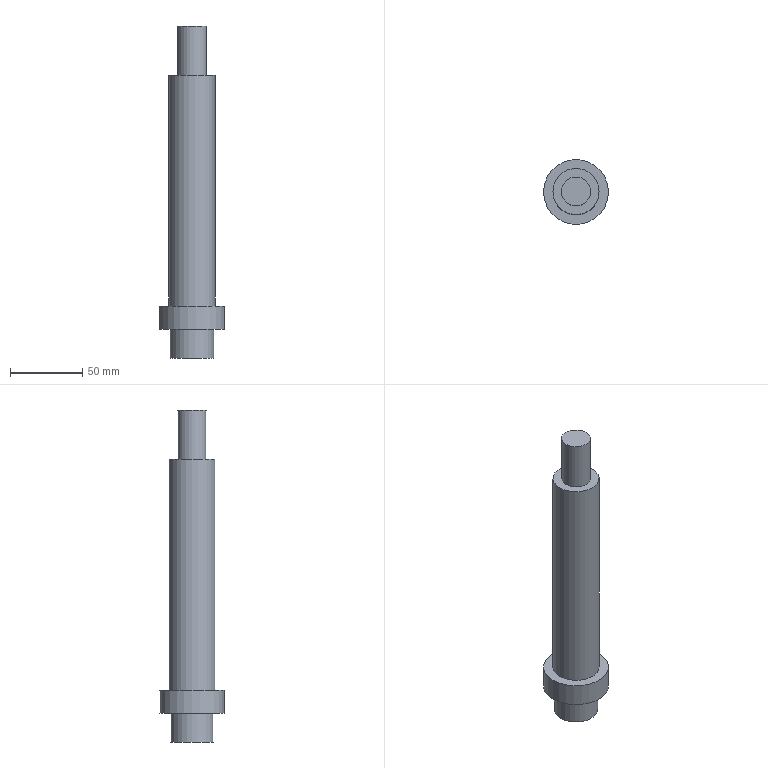Part | NX | features solid 2 | 1 solid | 9 faces | box 45 x 45 x 230 mm | volume 178945 mm3 | plane 5 | cylinder 4 | commonest cylinder face diameters 20 x1 30 x1 32 x1 45 x1
STEP:
#1=CARTESIAN_POINT('',(-305.,-95.,350.));
#2=VERTEX_POINT('',#1);
#3=CARTESIAN_POINT('',(-315.,-95.,350.));
#4=DIRECTION('',(0.,0.,1.));
#5=DIRECTION('',(1.,0.,0.));
#6=AXIS2_PLACEMENT_3D('',#3,#4,#5);
#7=CIRCLE('',#6,10.);
#8=EDGE_CURVE('',#2,#2,#7,.F.);
#9=ORIENTED_EDGE('',*,*,#8,.T.);
#10=EDGE_LOOP('',(#9));
#11=FACE_BOUND('',#10,.T.);
#12=CARTESIAN_POINT('',(-299.,-95.,350.));
#13=VERTEX_POINT('',#12);
#14=CARTESIAN_POINT('',(-315.,-95.,350.));
#15=DIRECTION('',(0.,0.,1.));
#16=DIRECTION('',(1.,0.,0.));
#17=AXIS2_PLACEMENT_3D('',#14,#15,#16);
#18=CIRCLE('',#17,16.);
#19=EDGE_CURVE('',#13,#13,#18,.T.);
#20=ORIENTED_EDGE('',*,*,#19,.T.);
#21=EDGE_LOOP('',(#20));
#22=FACE_BOUND('',#21,.T.);
#23=CARTESIAN_POINT('',(-315.,-95.,350.));
#24=DIRECTION('',(0.,0.,1.));
#25=DIRECTION('',(-1.,0.,0.));
#26=AXIS2_PLACEMENT_3D('',#23,#24,#25);
#27=PLANE('',#26);
#28=ADVANCED_FACE('',(#11,#22),#27,.T.);
#29=CARTESIAN_POINT('',(-331.,-95.,190.));
#30=VERTEX_POINT('',#29);
#31=CARTESIAN_POINT('',(-315.,-95.,190.));
#32=DIRECTION('',(0.,0.,-1.));
#33=DIRECTION('',(-1.,0.,0.));
#34=AXIS2_PLACEMENT_3D('',#31,#32,#33);
#35=CIRCLE('',#34,16.);
#36=EDGE_CURVE('',#30,#30,#35,.F.);
#37=ORIENTED_EDGE('',*,*,#36,.T.);
#38=EDGE_LOOP('',(#37));
#39=FACE_BOUND('',#38,.T.);
#40=ORIENTED_EDGE('',*,*,#19,.F.);
#41=EDGE_LOOP('',(#40));
#42=FACE_BOUND('',#41,.T.);
#43=CARTESIAN_POINT('',(-315.,-95.,430.));
#44=DIRECTION('',(0.,0.,-1.));
#45=DIRECTION('',(1.,0.,0.));
#46=AXIS2_PLACEMENT_3D('',#43,#44,#45);
#47=CYLINDRICAL_SURFACE('',#46,16.);
#48=ADVANCED_FACE('',(#39,#42),#47,.T.);
#49=CARTESIAN_POINT('',(-305.,-95.,384.));
#50=VERTEX_POINT('',#49);
#51=CARTESIAN_POINT('',(-315.,-95.,384.));
#52=DIRECTION('',(0.,0.,1.));
#53=DIRECTION('',(1.,0.,0.));
#54=AXIS2_PLACEMENT_3D('',#51,#52,#53);
#55=CIRCLE('',#54,10.);
#56=EDGE_CURVE('',#50,#50,#55,.T.);
#57=ORIENTED_EDGE('',*,*,#56,.T.);
#58=EDGE_LOOP('',(#57));
#59=FACE_BOUND('',#58,.T.);
#60=CARTESIAN_POINT('',(-315.,-95.,384.));
#61=DIRECTION('',(0.,0.,1.));
#62=DIRECTION('',(-1.,0.,0.));
#63=AXIS2_PLACEMENT_3D('',#60,#61,#62);
#64=PLANE('',#63);
#65=ADVANCED_FACE('',(#59),#64,.T.);
#66=ORIENTED_EDGE('',*,*,#56,.F.);
#67=EDGE_LOOP('',(#66));
#68=FACE_BOUND('',#67,.T.);
#69=ORIENTED_EDGE('',*,*,#8,.F.);
#70=EDGE_LOOP('',(#69));
#71=FACE_BOUND('',#70,.T.);
#72=CARTESIAN_POINT('',(-315.,-95.,430.));
#73=DIRECTION('',(0.,0.,1.));
#74=DIRECTION('',(-1.,0.,0.));
#75=AXIS2_PLACEMENT_3D('',#72,#73,#74);
#76=CYLINDRICAL_SURFACE('',#75,10.);
#77=ADVANCED_FACE('',(#68,#71),#76,.T.);
#78=CARTESIAN_POINT('',(-300.,-95.,174.));
#79=VERTEX_POINT('',#78);
#80=CARTESIAN_POINT('',(-315.,-95.,174.));
#81=DIRECTION('',(0.,0.,1.));
#82=DIRECTION('',(1.,0.,0.));
#83=AXIS2_PLACEMENT_3D('',#80,#81,#82);
#84=CIRCLE('',#83,15.);
#85=EDGE_CURVE('',#79,#79,#84,.T.);
#86=ORIENTED_EDGE('',*,*,#85,.T.);
#87=EDGE_LOOP('',(#86));
#88=FACE_BOUND('',#87,.T.);
#89=CARTESIAN_POINT('',(-337.5,-95.,174.));
#90=VERTEX_POINT('',#89);
#91=CARTESIAN_POINT('',(-315.,-95.,174.));
#92=DIRECTION('',(0.,0.,-1.));
#93=DIRECTION('',(-1.,0.,0.));
#94=AXIS2_PLACEMENT_3D('',#91,#92,#93);
#95=CIRCLE('',#94,22.5);
#96=EDGE_CURVE('',#90,#90,#95,.T.);
#97=ORIENTED_EDGE('',*,*,#96,.T.);
#98=EDGE_LOOP('',(#97));
#99=FACE_BOUND('',#98,.T.);
#100=CARTESIAN_POINT('',(-315.,-95.,174.));
#101=DIRECTION('',(0.,0.,-1.));
#102=DIRECTION('',(1.,0.,0.));
#103=AXIS2_PLACEMENT_3D('',#100,#101,#102);
#104=PLANE('',#103);
#105=ADVANCED_FACE('',(#88,#99),#104,.T.);
#106=ORIENTED_EDGE('',*,*,#36,.F.);
#107=EDGE_LOOP('',(#106));
#108=FACE_BOUND('',#107,.T.);
#109=CARTESIAN_POINT('',(-292.5,-95.,190.));
#110=VERTEX_POINT('',#109);
#111=CARTESIAN_POINT('',(-315.,-95.,190.));
#112=DIRECTION('',(0.,0.,1.));
#113=DIRECTION('',(1.,0.,0.));
#114=AXIS2_PLACEMENT_3D('',#111,#112,#113);
#115=CIRCLE('',#114,22.5);
#116=EDGE_CURVE('',#110,#110,#115,.T.);
#117=ORIENTED_EDGE('',*,*,#116,.T.);
#118=EDGE_LOOP('',(#117));
#119=FACE_BOUND('',#118,.T.);
#120=CARTESIAN_POINT('',(-315.,-95.,190.));
#121=DIRECTION('',(0.,0.,1.));
#122=DIRECTION('',(-1.,0.,0.));
#123=AXIS2_PLACEMENT_3D('',#120,#121,#122);
#124=PLANE('',#123);
#125=ADVANCED_FACE('',(#108,#119),#124,.T.);
#126=ORIENTED_EDGE('',*,*,#96,.F.);
#127=EDGE_LOOP('',(#126));
#128=FACE_BOUND('',#127,.T.);
#129=ORIENTED_EDGE('',*,*,#116,.F.);
#130=EDGE_LOOP('',(#129));
#131=FACE_BOUND('',#130,.T.);
#132=CARTESIAN_POINT('',(-315.,-95.,190.));
#133=DIRECTION('',(0.,0.,-1.));
#134=DIRECTION('',(1.,0.,0.));
#135=AXIS2_PLACEMENT_3D('',#132,#133,#134);
#136=CYLINDRICAL_SURFACE('',#135,22.5);
#137=ADVANCED_FACE('',(#128,#131),#136,.T.);
#138=CARTESIAN_POINT('',(-330.,-95.,154.));
#139=VERTEX_POINT('',#138);
#140=CARTESIAN_POINT('',(-315.,-95.,154.));
#141=DIRECTION('',(0.,0.,-1.));
#142=DIRECTION('',(-1.,0.,0.));
#143=AXIS2_PLACEMENT_3D('',#140,#141,#142);
#144=CIRCLE('',#143,15.);
#145=EDGE_CURVE('',#139,#139,#144,.T.);
#146=ORIENTED_EDGE('',*,*,#145,.T.);
#147=EDGE_LOOP('',(#146));
#148=FACE_BOUND('',#147,.T.);
#149=CARTESIAN_POINT('',(-315.,-95.,154.));
#150=DIRECTION('',(0.,0.,-1.));
#151=DIRECTION('',(1.,0.,0.));
#152=AXIS2_PLACEMENT_3D('',#149,#150,#151);
#153=PLANE('',#152);
#154=ADVANCED_FACE('',(#148),#153,.T.);
#155=ORIENTED_EDGE('',*,*,#145,.F.);
#156=EDGE_LOOP('',(#155));
#157=FACE_BOUND('',#156,.T.);
#158=ORIENTED_EDGE('',*,*,#85,.F.);
#159=EDGE_LOOP('',(#158));
#160=FACE_BOUND('',#159,.T.);
#161=CARTESIAN_POINT('',(-315.,-95.,174.));
#162=DIRECTION('',(0.,0.,-1.));
#163=DIRECTION('',(1.,0.,0.));
#164=AXIS2_PLACEMENT_3D('',#161,#162,#163);
#165=CYLINDRICAL_SURFACE('',#164,15.);
#166=ADVANCED_FACE('',(#157,#160),#165,.T.);
#167=CLOSED_SHELL('',(#28,#48,#65,#77,#105,#125,#137,#154,#166));
#168=MANIFOLD_SOLID_BREP('',#167);
#169=(LENGTH_UNIT()NAMED_UNIT(*)SI_UNIT(.MILLI.,.METRE.));
#170=UNCERTAINTY_MEASURE_WITH_UNIT(LENGTH_MEASURE(0.00001),#169,'','');
#171=(NAMED_UNIT(*)PLANE_ANGLE_UNIT()SI_UNIT($,.RADIAN.));
#172=(NAMED_UNIT(*)SI_UNIT($,.STERADIAN.)SOLID_ANGLE_UNIT());
#173=(GEOMETRIC_REPRESENTATION_CONTEXT(3)GLOBAL_UNCERTAINTY_ASSIGNED_CONTEXT((#170))GLOBAL_UNIT_ASSIGNED_CONTEXT((#169,#171,#172))REPRESENTATION_CONTEXT('',''));
#174=ADVANCED_BREP_SHAPE_REPRESENTATION('',(#168),#173);